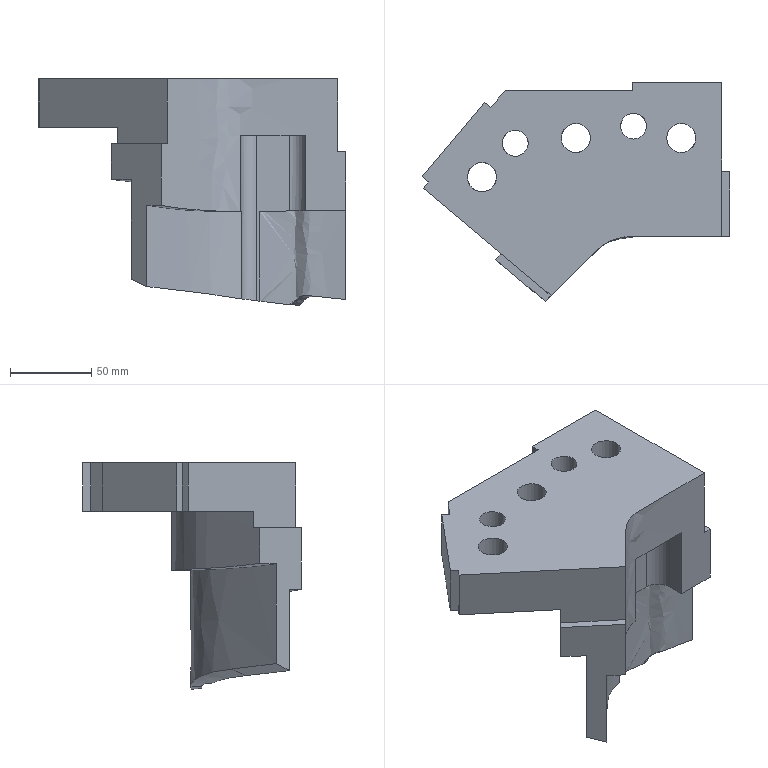Part | NX | features solid 2 | 1 solid | 51 faces | box 189.808 x 134.942 x 139.792 mm | volume 740828 mm3 | plane 23 | spline 18 | cylinder 10 | commonest cylinder face diameters 18 x3 26 x3 16 x2 20 x2